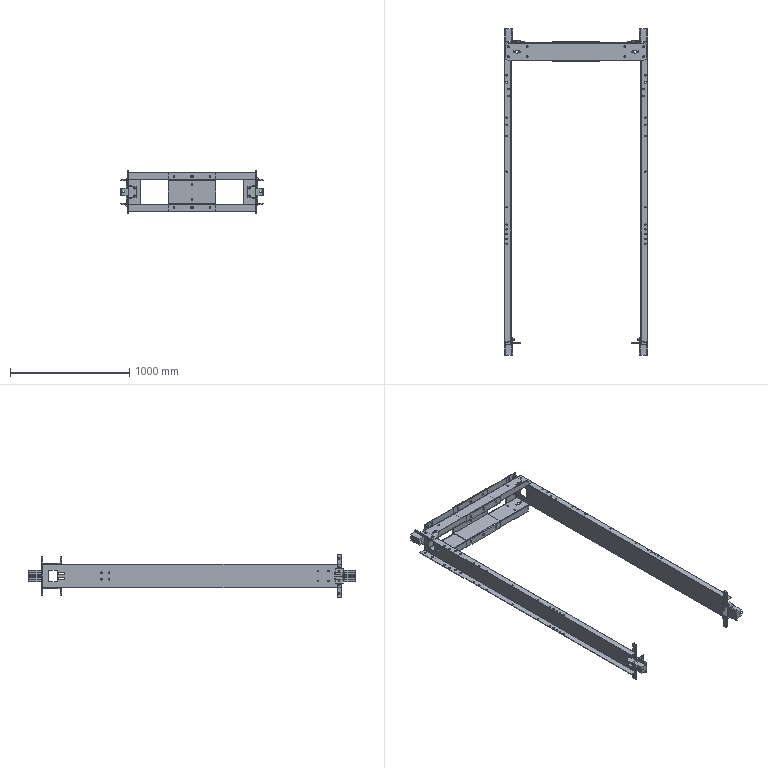Part | 18 solids | 876 faces | box 1204 x 2739 x 360 mm | volume 13859284 mm3 | cylinder 450 | plane 418 | spline 8 | commonest cylinder face diameters 14 x222 11 x80 13 x40 12 x24 12.5 x16 20 x12